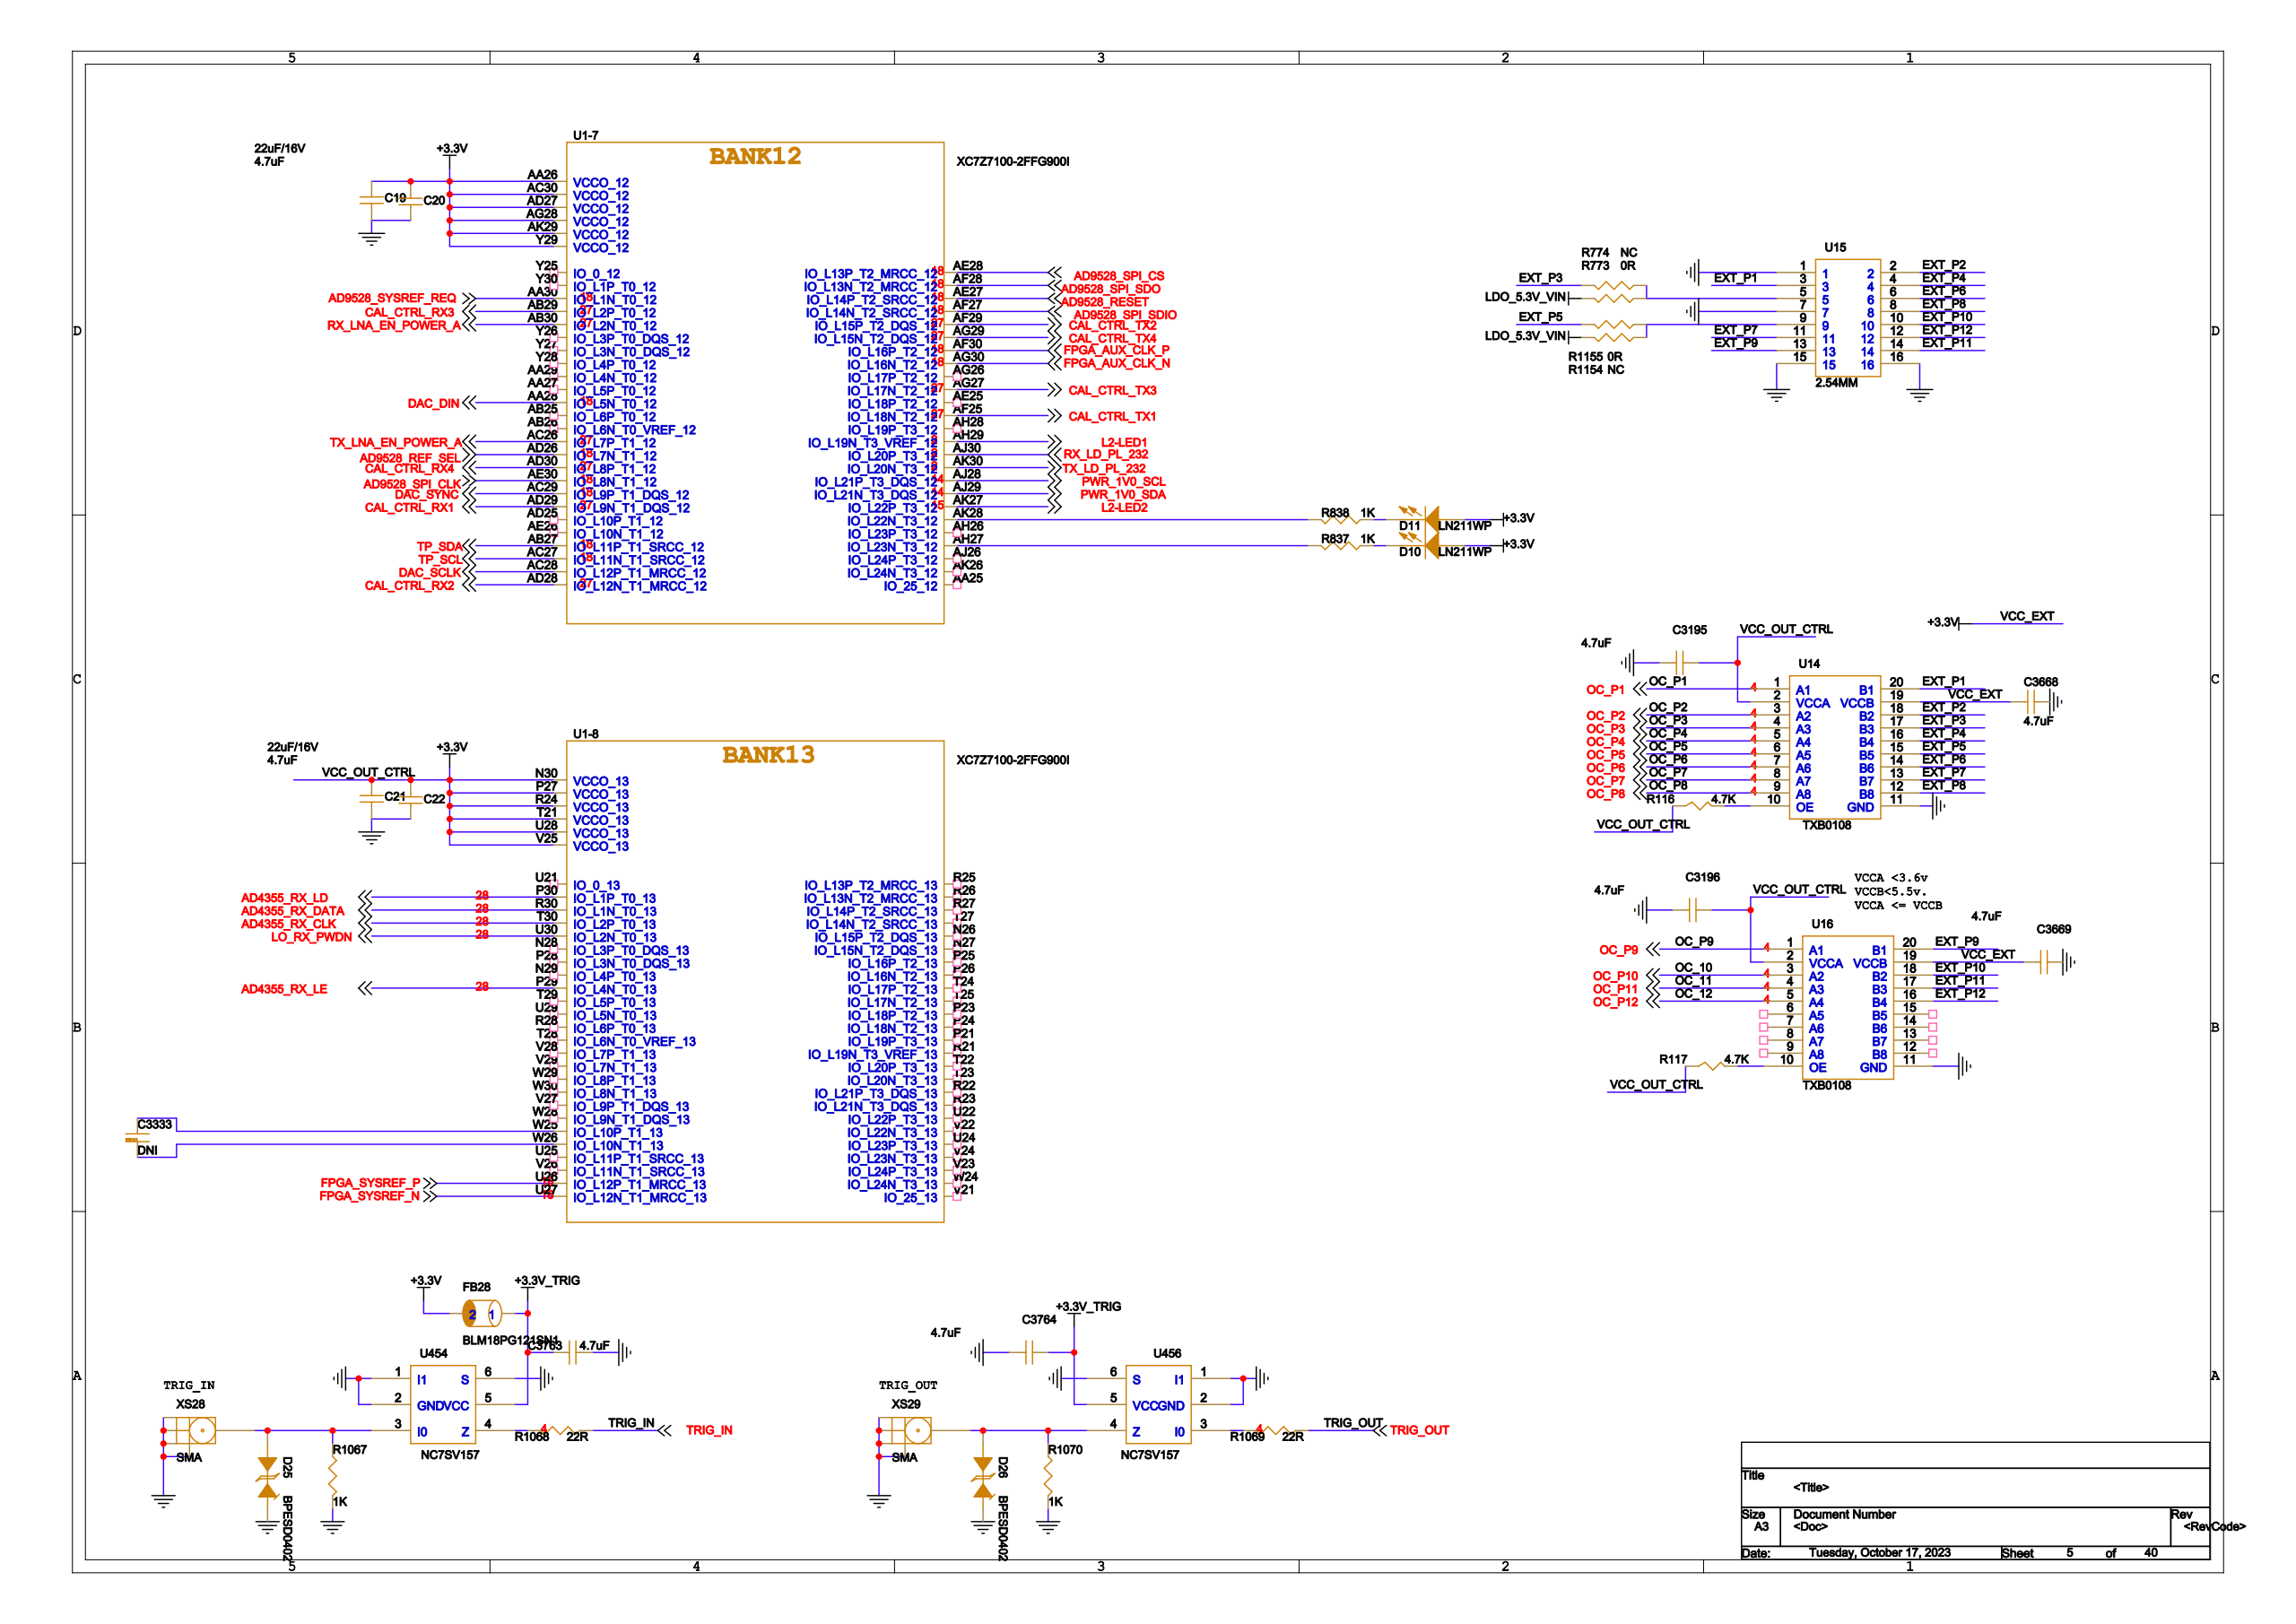Circuit board | Cadence Allegro | 1793 parts | 1223 nets | one sheet of the schematic
Parts on this sheet (reference | value | footprint):
C3195 | 4.7uF | C0402
C3196 | 4.7uF | C0402
C3333 | DNI | C0402
C3668 | 4.7uF | C0402
C3669 | 4.7uF | C0402
C3763 | 4.7uF | C0402
C3764 | 4.7uF | C0402
D10 | LN211WP | D0603
D11 | LN211WP | D0603
D25 | BPESD0402 | C0402
D26 | BPESD0402 | C0402
FB28 | BLM18PG121SN1 | FB0603
R116 | 4.7K | R0402
R117 | 4.7K | R0402
R773 | 0R | R0402
R774 | NC | R0402
R837 | 1K | R0402
R838 | 1K | R0402
R1067 | 1K | R0402
R1068 | 22R | R0402
R1069 | 22R | R0402
R1070 | 1K | R0402
R1154 | NC | R0402
R1155 | 0R | R0402
U14 | TXB0108 | LC-TSSOP-20
U15 | 2.54MM | DIP2X8_2_54
U16 | TXB0108 | LC-TSSOP-20
U454 | NC7SV157 | SC70-6
U456 | NC7SV157 | SC70-6
XS28 | SMA | SMA_5X5MM
XS29 | SMA | SMA_5X5MM
Nets of these parts (net: part-pin ...):
GND: C3195-2 C3196-2 C3668-1 C3669-1 C3763-2 C3764-2 D25-2 D26-2 R1067-1 R1070-1 U14-11 U15-1 U15-7 U15-15 U15-16 U16-11 U454-1 U454-2 U454-6 U456-1 U456-2 U456-6 XS28-2 XS28-3 XS28-4 XS28-5 XS29-2 XS29-3 XS29-4 XS29-5
EXT_P10: U15-10 U16-18
EXT_P7: U14-13 U15-11
EXT_P12: U15-12 U16-16
EXT_P9: U15-13 U16-20
EXT_P11: U15-14 U16-17
EXT_P2: U14-18 U15-2
EXT_P1: U14-20 U15-3
EXT_P4: U14-16 U15-4
N18613978: R773-2 R774-2 U15-5
EXT_P6: U14-14 U15-6
EXT_P8: U14-12 U15-8
N18613985: R1154-2 R1155-2 U15-9
N17943174: D25-1 R1067-2 U454-3 XS28-1
N17942315: D26-1 R1070-2 U456-4 XS29-1
+3.3V: C3195-1 C3196-1 C3668-2 C3669-2 D10-1 D11-1 FB28-2 R116-1 R117-1 U14-2 U14-19 U16-2 U16-19
LDO_5.3V_VIN: R773-1 R1154-1
+3.3V_TRIG: C3763-1 C3764-1 FB28-1 U454-5 U456-5
N17943182: R1068-1 U454-4
TRIG_IN: R1068-2
N17942323: R1069-1 U456-3
TRIG_OUT: R1069-2
EXT_P3: R774-1 U14-17
OC_P1: U14-1
OC_P2: U14-3
OC_P3: U14-4
OC_P4: U14-5
OC_P5: U14-6
OC_P6: U14-7
OC_P7: U14-8
OC_P8: U14-9
EXT_P5: R1155-1 U14-15
N17941770: R116-2 U14-10
OC_P9: U16-1
OC_P10: U16-3
OC_P11: U16-4
OC_P12: U16-5
N17941899: R117-2 U16-10
N17940275: C3333-1
N17940258: C3333-2
N18841180: D10-2 R837-2
N18841152: D11-2 R838-2
N18841498: R837-1
N18841148: R838-1